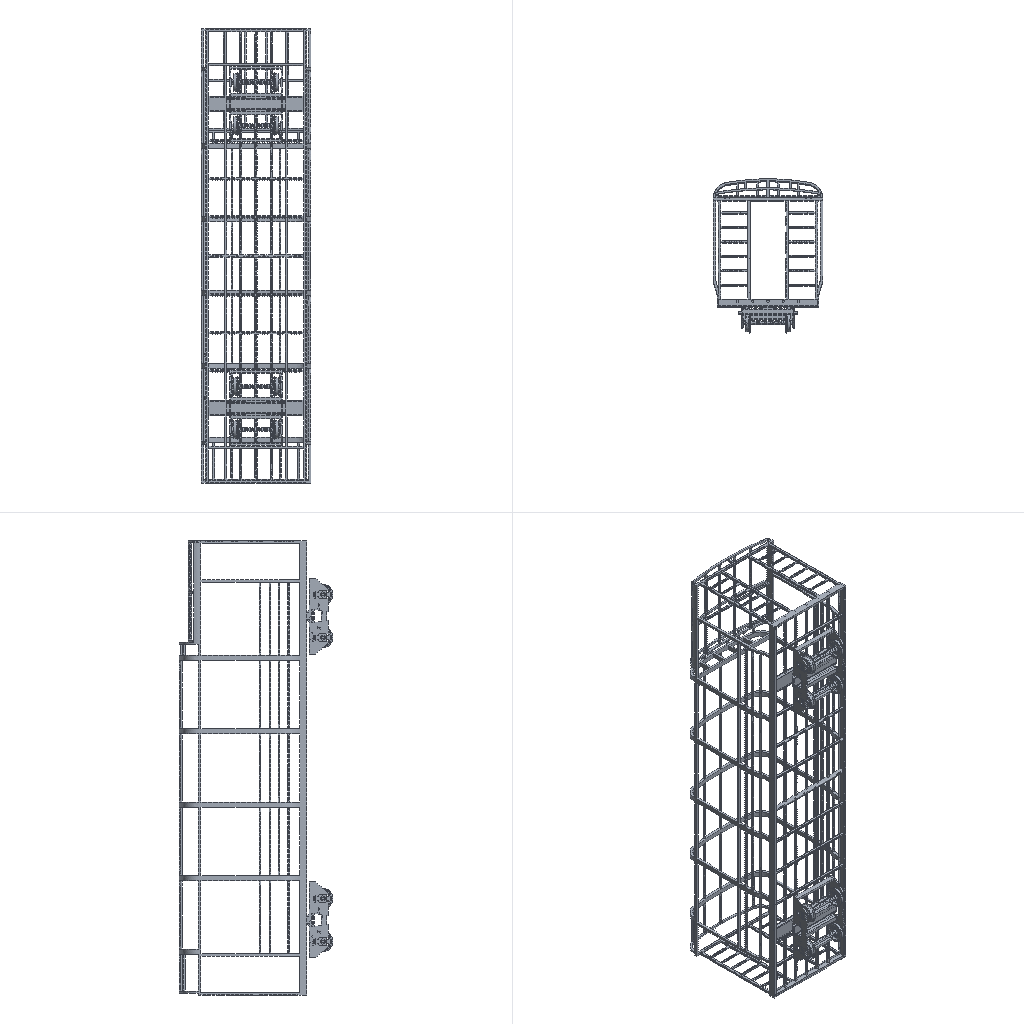Simulation study | ansys workbench
Set-up summary:
category,name,step,type,value,unit,region
solver,ansys_workbench
units,mm-N-s-tonne (MPa),,stated,"/units,MPA"
analysis,LS1,,static
load_step,LS1,LS1,static,nsubst=1; time=1
mesh,nodes,,,844920
mesh,elements,,,484857
element_type,SOLID187,,,440747
element_type,CONTA174,,,29118
element_type,TARGE170,,,10972
element_type,SOLID186,,,4020
material,Structural Steel,,E,200000,tonne s^-2 mm^-1
material,Structural Steel,,nu,0.3
material,Structural Steel,,density,7.85e-09,tonne mm^-3
material,Structural Steel,,conductivity,60.5,tonne mm s^-3 C^-1
material,Structural Steel,,specific_heat,4.34e+08,mm^2 s^-2 C^-1
material,Structural Steel,,cte,1.2e-05,C^-1
material,Structural Steel,,permeability,10000
material,Structural Steel,,resistivity,0.00017,ohm mm
load,,LS1,moment,"2.62e+06 [dir=(1, 0, 0) n=12]",,all
load,,LS1,force,"4284 [dir=(-1, 0, 0) n=3]",,all
load,ACEL,LS1,gravity (ACEL; gravity acts opposite),"9810.13 [dir=(0.02664, -0.9996, 0)]",,all
bc,Constant Zero Displacement X,model,fixed,[dofs=UX],,_DISPZEROUX
bc,Constant Zero Displacement Y,model,fixed,[dofs=UY],,_DISPZEROUY
bc,Constant Zero Displacement Z,model,fixed,[dofs=UZ],,_DISPZEROUZ
contact,Contact Region 10,,bonded (always),element=CONTA174
contact,Contact Region 11,,bonded (always),element=CONTA174
contact,Contact Region 12,,bonded (always),element=CONTA174
contact,Contact Region 13,,bonded (always),element=CONTA174
contact,Contact Region 14,,bonded (always),element=CONTA174
contact,Contact Region 15,,bonded (always),element=CONTA174
contact,Contact Region 16,,bonded (always),element=CONTA174
contact,Contact Region 17,,bonded (always),element=CONTA174
contact,Contact Region 18,,bonded (always),element=CONTA174
contact,Contact Region 19,,bonded (always),element=CONTA174
contact,Contact Region 20,,bonded (always),element=CONTA174
contact,Contact Region 21,,bonded (always),element=CONTA174
contact,Contact Region 22,,bonded (always),element=CONTA174
contact,Contact Region 23,,bonded (always),element=CONTA174
contact,Contact Region 24,,bonded (always),element=CONTA174
contact,Contact Region 25,,bonded (always),element=CONTA174
contact,Contact Region 26,,bonded (always),element=CONTA174
contact,Contact Region 27,,bonded (always),element=CONTA174
contact,Contact Region 28,,bonded (always),element=CONTA174
contact,Contact Region 29,,bonded (always),element=CONTA174
contact,Contact Region 30,,bonded (always),element=CONTA174
contact,Contact Region 31,,bonded (always),element=CONTA174
contact,Contact Region 32,,bonded (always),element=CONTA174
contact,Contact Region 33,,bonded (always),element=CONTA174
contact,Contact Region 34,,bonded (always),element=CONTA174
contact,Contact Region 35,,bonded (always),element=CONTA174
contact,Contact Region 36,,bonded (always),element=CONTA174
contact,Contact Region 37,,bonded (always),element=CONTA174
contact,Contact Region 38,,bonded (always),element=CONTA174
contact,Contact Region 39,,bonded (always),element=CONTA174
contact,Contact Region 40,,bonded (always),element=CONTA174
contact,Contact Region 41,,bonded (always),element=CONTA174
contact,Contact Region 42,,bonded (always),element=CONTA174
contact,Contact Region 43,,bonded (always),element=CONTA174
contact,Contact Region 44,,bonded (always),element=CONTA174
contact,Contact Region 45,,bonded (always),element=CONTA174
contact,Contact Region 46,,bonded (always),element=CONTA174
contact,Contact Region 47,,bonded (always),element=CONTA174
contact,Contact Region 48,,bonded (always),element=CONTA174
contact,Contact Region 49,,bonded (always),element=CONTA174
contact,Contact Region 50,,bonded (always),element=CONTA174
contact,Contact Region 51,,bonded (always),element=CONTA174
contact,Contact Region 52,,bonded (always),element=CONTA174
contact,Contact Region 53,,bonded (always),element=CONTA174
contact,Contact Region 54,,bonded (always),element=CONTA174
contact,Contact Region 55,,bonded (always),element=CONTA174
contact,Contact Region 56,,bonded (always),element=CONTA174
contact,Contact Region 57,,bonded (always),element=CONTA174
contact,Contact Region 58,,bonded (always),element=CONTA174
contact,Contact Region 59,,bonded (always),element=CONTA174
contact,Contact Region 60,,bonded (always),element=CONTA174
contact,Contact Region 61,,bonded (always),element=CONTA174
contact,Contact Region 62,,bonded (always),element=CONTA174
contact,Contact Region 63,,bonded (always),element=CONTA174
contact,Contact Region 64,,bonded (always),element=CONTA174
contact,Contact Region 65,,bonded (always),element=CONTA174
contact,Contact Region 66,,bonded (always),element=CONTA174
contact,Contact Region 67,,bonded (always),element=CONTA174
contact,Contact Region 68,,bonded (always),element=CONTA174
contact,Contact Region 69,,bonded (always),element=CONTA174
contact,Contact Region 70,,bonded (always),element=CONTA174
contact,Contact Region 71,,bonded (always),element=CONTA174
contact,Contact Region 72,,bonded (always),element=CONTA174
contact,Contact Region 73,,bonded (always),element=CONTA174
contact,Contact Region 74,,bonded (always),element=CONTA174
contact,Contact Region 75,,bonded (always),element=CONTA174
contact,Contact Region 76,,bonded (always),element=CONTA174
contact,Contact Region 77,,bonded (always),element=CONTA174
contact,Contact Region 78,,bonded (always),element=CONTA174
contact,Contact Region 79,,bonded (always),element=CONTA174
contact,Contact Region 80,,bonded (always),element=CONTA174
contact,Contact Region 81,,bonded (always),element=CONTA174
contact,Contact Region 82,,bonded (always),element=CONTA174
contact,Contact Region 83,,bonded (always),element=CONTA174
contact,Contact Region 84,,bonded (always),element=CONTA174
contact,Contact Region 85,,bonded (always),element=CONTA174
contact,Contact Region 86,,bonded (always),element=CONTA174
contact,Contact Region 87,,bonded (always),element=CONTA174
contact,Contact Region 88,,bonded (always),element=CONTA174
contact,Contact Region 89,,bonded (always),element=CONTA174
contact,Contact Region 90,,bonded (always),element=CONTA174
contact,Contact Region 91,,bonded (always),element=CONTA174
contact,Contact Region 92,,bonded (always),element=CONTA174
contact,Contact Region 93,,bonded (always),element=CONTA174
contact,Contact Region 94,,bonded (always),element=CONTA174
contact,Contact Region 95,,bonded (always),element=CONTA174
contact,Contact Region 96,,bonded (always),element=CONTA174
contact,Contact Region 97,,bonded (always),element=CONTA174
contact,Contact Region 98,,bonded (always),element=CONTA174
contact,Contact Region 99,,bonded (always),element=CONTA174
contact,Contact Region 100,,bonded (always),element=CONTA174
contact,Contact Region 101,,bonded (always),element=CONTA174
contact,Contact Region 102,,bonded (always),element=CONTA174
contact,Contact Region 103,,bonded (always),element=CONTA174
contact,Contact Region 104,,bonded (always),element=CONTA174
contact,Contact Region 105,,bonded (always),element=CONTA174
contact,Contact Region 106,,bonded (always),element=CONTA174
contact,Contact Region 107,,bonded (always),element=CONTA174
contact,Contact Region 108,,bonded (always),element=CONTA174
contact,Contact Region 109,,bonded (always),element=CONTA174
contact,Contact Region 110,,bonded (always),element=CONTA174
contact,Contact Region 111,,bonded (always),element=CONTA174
contact,Contact Region 112,,bonded (always),element=CONTA174
contact,Contact Region 113,,bonded (always),element=CONTA174
contact,Contact Region 114,,bonded (always),element=CONTA174
contact,Contact Region 115,,bonded (always),element=CONTA174
contact,Contact Region 116,,bonded (always),element=CONTA174
contact,Contact Region 117,,bonded (always),element=CONTA174
contact,Contact Region 118,,bonded (always),element=CONTA174
contact,Contact Region 119,,bonded (always),element=CONTA174
contact,Contact Region 120,,bonded (always),element=CONTA174
contact,contact 112,,bonded (always),element=CONTA174
contact,contact 113,,bonded (always),element=CONTA174
contact,contact 114,,bonded (always),element=CONTA174
contact,contact 115,,bonded (always),element=CONTA174
contact,contact 116,,bonded (always),element=CONTA174
contact,contact 117,,bonded (always),element=CONTA174
contact,contact 118,,bonded (always),element=CONTA174
named_set,_DISPZEROUX,,node,2976
named_set,_DISPZEROUY,,node,2976
named_set,_DISPZEROUZ,,node,1488
Ansys APDL input file, long lists of numbers shortened:
/batch
/config,noeldb,1     ! force off writing results to database
*get,_wallstrt,active,,time,wall
! ANSYS input file written by Workbench version 2021 R1
! File used for geometry attach:
/title,_______--____ 2 (C5)
! ****** Begin Custom Load Command Snippet ******
/COM, ACT Extensions:
/COM,     LSDYNA, 2021.1
/COM,
! ****** End   Custom Load Command Snippet ******
*DIM,_wb_ProjectScratch_dir,string,248
_wb_ProjectScratch_dir(1) = ''
*DIM,_wb_SolverFiles_dir,string,248
_wb_SolverFiles_dir(1) = ''
*DIM,_wb_userfiles_dir,string,248
_wb_userfiles_dir(1) = ''
/com,--- Data in consistent NMM units. See Solving Units in the help system for more information.
/units,MPA
/nopr
/wb,file,start              !  signify a WB generated input file
/prep7
! Turn off shape checking because checks already performed inside WB mesher.
! See help system for more information.
SHPP,OFF,,NOWARN
/nolist
etcon,set             ! allow ANSYS to choose best KEYOP's for 180x elements, resets any applicable keyopt to MAPDL defaults
/com,*********** Nodes for the whole assembly ***********
nblock,3,,929390
(1i9,3e20.9e3)
        1     5.000000000E+02    -2.700000000E+02     8.500000000E+01
! (844899 more lines like these left out)
-1
/com,*********** Nodes for all Remote Points ***********
nblock,3
(1i9,3e20.9e3)
   844901     0.000000000E+00    -4.570000000E+02     1.250000000E+03
! (19 more lines like these left out)
-1
/wb,elem,start            !  set before creation of elements
/com,*********** Elements for Body 1 "____-0|NONE" ***********
et,1,187
eblock,19,solid,,219008
(19i9)
        1        1        1        1        0        0        0        0       10        0   225760   496373   499028   502293   501893   835194   841376   835201   835199
! (438015 more lines like these left out)
-1
/com,*********** Elements for Body 2 "______|NONE" ***********
et,2,186
keyo,2,2,1          ! set full integration on SOLID186
eblock,19,solid,,316
(19i9)
        2        2        2        2        0        0        0        0       20        0      914     6556     6586     6589     6565     6931     6901     6898     6922
! (631 more lines like these left out)
-1
/com,*********** Elements for Body 3 "______|NONE[2]" ***********
et,3,186
keyo,3,2,1          ! set full integration on SOLID186
eblock,19,solid,,316
(19i9)
        3        3        3        3        0        0        0        0       20        0     1663    12147    12177    12180    12156    12522    12492    12489    12513
! (631 more lines like these left out)
-1
/com,*********** Elements for Body 4 "______|NONE[3]" ***********
et,4,186
keyo,4,2,1          ! set full integration on SOLID186
eblock,19,solid,,420
(19i9)
        4        4        4        4        0        0        0        0       20        0     1243     9304     9447     9466     9364     9345     9446     9485     9365
! (839 more lines like these left out)
-1
/com,*********** Elements for Body 5 "______|NONE[4]" ***********
et,5,186
keyo,5,2,1          ! set full integration on SOLID186
eblock,19,solid,,420
(19i9)
        5        5        5        5        0        0        0        0       20        0      481     3579     3722     3741     3639     3620     3721     3760     3640
! (839 more lines like these left out)
-1
! (55 more sections like these left out)
/wb,elem,end               !  done creating elements
/com,*********** Send User Defined Coordinate System(s) ***********
csys,0
toffst,273.15,  ! Temperature offset from absolute zero
/com,*********** Set Reference Temperature ***********
tref,22.
/wb,mat,start              !  starting to send materials
/com,*********** Send Materials ***********
Temperature = 'TEMP' ! Temperature
MP,DENS,1,7.85e-09,	! tonne mm^-3
MP,ALPX,1,1.2e-05,	! C^-1
MP,C,1,434000000,	! mm^2 s^-2 C^-1
MP,KXX,1,60.5,	! tonne mm s^-3 C^-1
MP,RSVX,1,0.00017,	! ohm mm
MP,EX,1,200000,	! tonne s^-2 mm^-1
MP,NUXY,1,0.3,
MP,MURX,1,10000,
Temperature = 'TEMP' ! Temperature
MP,DENS,2,7.85e-09,	! tonne mm^-3
MP,ALPX,2,1.2e-05,	! C^-1
MP,C,2,434000000,	! mm^2 s^-2 C^-1
MP,KXX,2,60.5,	! tonne mm s^-3 C^-1
MP,RSVX,2,0.00017,	! ohm mm
MP,EX,2,200000,	! tonne s^-2 mm^-1
MP,NUXY,2,0.3,
MP,MURX,2,10000,
Temperature = 'TEMP' ! Temperature
MP,DENS,3,7.85e-09,	! tonne mm^-3
MP,ALPX,3,1.2e-05,	! C^-1
MP,C,3,434000000,	! mm^2 s^-2 C^-1
MP,KXX,3,60.5,	! tonne mm s^-3 C^-1
MP,RSVX,3,0.00017,	! ohm mm
MP,EX,3,200000,	! tonne s^-2 mm^-1
MP,NUXY,3,0.3,
MP,MURX,3,10000,
Temperature = 'TEMP' ! Temperature
MP,DENS,4,7.85e-09,	! tonne mm^-3
MP,ALPX,4,1.2e-05,	! C^-1
MP,C,4,434000000,	! mm^2 s^-2 C^-1
MP,KXX,4,60.5,	! tonne mm s^-3 C^-1
MP,RSVX,4,0.00017,	! ohm mm
MP,EX,4,200000,	! tonne s^-2 mm^-1
MP,NUXY,4,0.3,
MP,MURX,4,10000,
Temperature = 'TEMP' ! Temperature
MP,DENS,5,7.85e-09,	! tonne mm^-3
MP,ALPX,5,1.2e-05,	! C^-1
MP,C,5,434000000,	! mm^2 s^-2 C^-1
MP,KXX,5,60.5,	! tonne mm s^-3 C^-1
MP,RSVX,5,0.00017,	! ohm mm
MP,EX,5,200000,	! tonne s^-2 mm^-1
MP,NUXY,5,0.3,
MP,MURX,5,10000,
Temperature = 'TEMP' ! Temperature
MP,DENS,6,7.85e-09,	! tonne mm^-3
MP,ALPX,6,1.2e-05,	! C^-1
MP,C,6,434000000,	! mm^2 s^-2 C^-1
MP,KXX,6,60.5,	! tonne mm s^-3 C^-1
MP,RSVX,6,0.00017,	! ohm mm
MP,EX,6,200000,	! tonne s^-2 mm^-1
MP,NUXY,6,0.3,
MP,MURX,6,10000,
Temperature = 'TEMP' ! Temperature
MP,DENS,7,7.85e-09,	! tonne mm^-3
MP,ALPX,7,1.2e-05,	! C^-1
MP,C,7,434000000,	! mm^2 s^-2 C^-1
MP,KXX,7,60.5,	! tonne mm s^-3 C^-1
MP,RSVX,7,0.00017,	! ohm mm
MP,EX,7,200000,	! tonne s^-2 mm^-1
MP,NUXY,7,0.3,
MP,MURX,7,10000,
Temperature = 'TEMP' ! Temperature
MP,DENS,8,7.85e-09,	! tonne mm^-3
MP,ALPX,8,1.2e-05,	! C^-1
MP,C,8,434000000,	! mm^2 s^-2 C^-1
MP,KXX,8,60.5,	! tonne mm s^-3 C^-1
MP,RSVX,8,0.00017,	! ohm mm
MP,EX,8,200000,	! tonne s^-2 mm^-1
MP,NUXY,8,0.3,
MP,MURX,8,10000,
Temperature = 'TEMP' ! Temperature
MP,DENS,9,7.85e-09,	! tonne mm^-3
MP,ALPX,9,1.2e-05,	! C^-1
MP,C,9,434000000,	! mm^2 s^-2 C^-1
MP,KXX,9,60.5,	! tonne mm s^-3 C^-1
MP,RSVX,9,0.00017,	! ohm mm
MP,EX,9,200000,	! tonne s^-2 mm^-1
! (461 more lines like these left out)
/wb,mat,end                !  done sending materials
!************************* Model Summary ********************
!____-0|NONE,	结构钢,	matid,	1
!______|NONE,	结构钢,	matid,	2
!______|NONE[2],	结构钢,	matid,	3
! (59 more lines like these left out)
*get,_xmin,node,,mnloc,x
*get,_ymin,node,,mnloc,y
*get,_zmin,node,,mnloc,z
*get,_xmax,node,,mxloc,x
*get,_ymax,node,,mxloc,y
*get,_zmax,node,,mxloc,z
_ASMDIAG=(_xmax-_xmin)*(_xmax-_xmin)+(_ymax-_ymin)*(_ymax-_ymin)+(_zmax-_zmin)*(_zmax-_zmin)
_ASMDIAG=SQRT(_ASMDIAG)
/wb,contact,start          !  starting to send contact
/com,*********** Create Contact "接触区域 10" ***********
/com,            Real Constant Set For Above Contact Is 62 & 61
*set,tid,62
*set,cid,61
r,tid
r,cid
et,tid,170
et,cid,174
eblock,10,,,42
(15i9)
   662848       62       62       62        0     6714     6723     6734     6734     7990     8015     6734     7992
! (41 more lines like these left out)
-1
eblock,10,,,42
(15i9)
   662890       61       61       61        0     6714     6723     6734     6734     7990     8015     6734     7992
! (41 more lines like these left out)
-1
eblock,10,,,21
(15i9)
   662932       61       62       61        0     9885    10045     9244     9244    11813    10203     9244    10202
! (20 more lines like these left out)
-1
eblock,10,,,21
(15i9)
   662953       62       61       62        0     9885    10045     9244     9244    11813    10203     9244    10202
! (20 more lines like these left out)
-1
keyo,cid,8,2               ! auto create asymmetric contact (from Program Controlled setting)
keyo,cid,10,0              ! adjust contact stiffness each NR iteration (from Program Controlled setting)
keyo,cid,12,5              ! bonded always
keyo,cid,18,1              ! small sliding turned on by application
keyo,cid,2,0               ! augmented Lagrange (from Program Controlled setting)
keyo,cid,4,0               ! on Gauss point (from Program Controlled setting)
keyo,cid,9,1               ! ignore initial gaps/penetration
keyo,cid,7,0               ! No Prediction
rmod,tid,3,10.      ! FKN
rmod,tid,5,0.       ! ICONT
rmod,tid,6,0.       ! PINB
rmod,tid,10,0.      ! CNOF
rmod,tid,12,0.      ! FKT
rmod,tid,36,14962   ! WB DSID
rmod,cid,3,10.      ! FKN
rmod,cid,5,0.       ! ICONT
rmod,cid,6,0.       ! PINB
rmod,cid,10,0.      ! CNOF
rmod,cid,12,0.      ! FKT
rmod,cid,36,14962   ! WB DSID
/com,*********** Create Contact "接触区域 11" ***********
/com,            Real Constant Set For Above Contact Is 64 & 63
*set,tid,64
*set,cid,63
r,tid
r,cid
et,tid,170
et,cid,174
eblock,10,,,48
(15i9)
   662974       64       64       64        0     6688     6733     6595     6595     7938     7613     6595     7610
! (47 more lines like these left out)
-1
eblock,10,,,48
(15i9)
   663022       63       63       63        0     6688     6733     6595     6595     7938     7613     6595     7610
! (47 more lines like these left out)
-1
eblock,10,,,21
(15i9)
   663070       63       64       63        0     3534     3522     3523     3523     4485     4484     3523     4488
! (20 more lines like these left out)
-1
eblock,10,,,21
(15i9)
   663091       64       63       64        0     3534     3522     3523     3523     4485     4484     3523     4488
! (20 more lines like these left out)
-1
keyo,cid,8,2               ! auto create asymmetric contact (from Program Controlled setting)
keyo,cid,10,0              ! adjust contact stiffness each NR iteration (from Program Controlled setting)
keyo,cid,12,5              ! bonded always
keyo,cid,18,1              ! small sliding turned on by application
keyo,cid,2,0               ! augmented Lagrange (from Program Controlled setting)
keyo,cid,4,0               ! on Gauss point (from Program Controlled setting)
keyo,cid,9,1               ! ignore initial gaps/penetration
keyo,cid,7,0               ! No Prediction
rmod,tid,3,10.      ! FKN
rmod,tid,5,0.       ! ICONT
rmod,tid,6,0.       ! PINB
rmod,tid,10,0.      ! CNOF
rmod,tid,12,0.      ! FKT
rmod,tid,36,14965   ! WB DSID
rmod,cid,3,10.      ! FKN
rmod,cid,5,0.       ! ICONT
rmod,cid,6,0.       ! PINB
rmod,cid,10,0.      ! CNOF
rmod,cid,12,0.      ! FKT
rmod,cid,36,14965   ! WB DSID
/com,*********** Create Contact "接触区域 12" ***********
/com,            Real Constant Set For Above Contact Is 66 & 65
*set,tid,66
*set,cid,65
r,tid
r,cid
et,tid,170
et,cid,174
eblock,10,,,16
(15i9)
   663112       66       66       66        0     6741     6708     6696     6709     7977     7955     7956     7980
! (15 more lines like these left out)
-1
eblock,10,,,16
(15i9)
   663128       65       65       65        0     6741     6708     6696     6709     7977     7955     7956     7980
! (15 more lines like these left out)
-1
eblock,10,,,12
(15i9)
   663144       65       66       65        0     1744     1745     1761     1756     2255     2259     2289     2257
! (11 more lines like these left out)
-1
eblock,10,,,12
(15i9)
   663156       66       65       66        0     1744     1745     1761     1756     2255     2259     2289     2257
! (11 more lines like these left out)
-1
keyo,cid,8,2               ! auto create asymmetric contact (from Program Controlled setting)
keyo,cid,10,0              ! adjust contact stiffness each NR iteration (from Program Controlled setting)
keyo,cid,12,5              ! bonded always
keyo,cid,18,1              ! small sliding turned on by application
keyo,cid,2,0               ! augmented Lagrange (from Program Controlled setting)
keyo,cid,4,0               ! on Gauss point (from Program Controlled setting)
keyo,cid,9,1               ! ignore initial gaps/penetration
keyo,cid,7,0               ! No Prediction
rmod,tid,3,10.      ! FKN
rmod,tid,5,0.       ! ICONT
rmod,tid,6,0.       ! PINB
rmod,tid,10,0.      ! CNOF
rmod,tid,12,0.      ! FKT
rmod,tid,36,14968   ! WB DSID
rmod,cid,3,10.      ! FKN
rmod,cid,5,0.       ! ICONT
rmod,cid,6,0.       ! PINB
rmod,cid,10,0.      ! CNOF
rmod,cid,12,0.      ! FKT
rmod,cid,36,14968   ! WB DSID
/com,*********** Create Contact "接触区域 13" ***********
/com,            Real Constant Set For Above Contact Is 68 & 67
*set,tid,68
*set,cid,67
r,tid
r,cid
et,tid,170
et,cid,174
eblock,10,,,15
(15i9)
   663168       68       68       68        0     6738     6691     6692     6739     7945     7944     7948     8042
! (14 more lines like these left out)
-1
eblock,10,,,15
(15i9)
   663183       67       67       67        0     6738     6691     6692     6739     7945     7944     7948     8042
! (14 more lines like these left out)
-1
eblock,10,,,12
(15i9)
   663198       67       68       67        0       21       16        4        5      549      517      515      519
! (11 more lines like these left out)
-1
eblock,10,,,12
(15i9)
   663210       68       67       68        0       21       16        4        5      549      517      515      519
! (11 more lines like these left out)
-1
keyo,cid,8,2               ! auto create asymmetric contact (from Program Controlled setting)
keyo,cid,10,0              ! adjust contact stiffness each NR iteration (from Program Controlled setting)
keyo,cid,12,5              ! bonded always
keyo,cid,18,1              ! small sliding turned on by application
keyo,cid,2,0               ! augmented Lagrange (from Program Controlled setting)
keyo,cid,4,0               ! on Gauss point (from Program Controlled setting)
keyo,cid,9,1               ! ignore initial gaps/penetration
keyo,cid,7,0               ! No Prediction
rmod,tid,3,10.      ! FKN
rmod,tid,5,0.       ! ICONT
rmod,tid,6,0.       ! PINB
rmod,tid,10,0.      ! CNOF
rmod,tid,12,0.      ! FKT
rmod,tid,36,14971   ! WB DSID
rmod,cid,3,10.      ! FKN
rmod,cid,5,0.       ! ICONT
rmod,cid,6,0.       ! PINB
rmod,cid,10,0.      ! CNOF
rmod,cid,12,0.      ! FKT
rmod,cid,36,14971   ! WB DSID
/com,*********** Create Contact "接触区域 14" ***********
/com,            Real Constant Set For Above Contact Is 70 & 69
*set,tid,70
*set,cid,69
r,tid
r,cid
et,tid,170
et,cid,174
eblock,10,,,33
(15i9)
   663222       70       70       70        0     7129     7127     7128     7133     8908     8907     8909     8911
! (32 more lines like these left out)
-1
eblock,10,,,33
(15i9)
   663255       69       69       69        0     7129     7127     7128     7133     8908     8907     8909     8911
! (32 more lines like these left out)
-1
eblock,10,,,170
(15i9)
   663288       69       70       69        0    17468    17488    17473    17473    26290    26306    17473    26287
! (169 more lines like these left out)
-1
eblock,10,,,170
(15i9)
   663458       70       69       70        0    17468    17488    17473    17473    26290    26306    17473    26287
! (169 more lines like these left out)
-1
keyo,cid,8,2               ! auto create asymmetric contact (from Program Controlled setting)
keyo,cid,10,0              ! adjust contact stiffness each NR iteration (from Program Controlled setting)
keyo,cid,12,5              ! bonded always
keyo,cid,18,1              ! small sliding turned on by application
keyo,cid,2,0               ! augmented Lagrange (from Program Controlled setting)
keyo,cid,4,0               ! on Gauss point (from Program Controlled setting)
keyo,cid,9,1               ! ignore initial gaps/penetration
keyo,cid,7,0               ! No Prediction
rmod,tid,3,10.      ! FKN
rmod,tid,5,0.       ! ICONT
rmod,tid,6,0.       ! PINB
rmod,tid,10,0.      ! CNOF
rmod,tid,12,0.      ! FKT
rmod,tid,36,14974   ! WB DSID
rmod,cid,3,10.      ! FKN
rmod,cid,5,0.       ! ICONT
rmod,cid,6,0.       ! PINB
rmod,cid,10,0.      ! CNOF
rmod,cid,12,0.      ! FKT
rmod,cid,36,14974   ! WB DSID
! (106 more sections like these left out)
/wb,contact,end            !  done creating contacts
/golist
/wb,load,start             !  starting to send loads
/com,******* Constant Zero Displacement X *******
CMBLOCK,_DISPZEROUX,NODE,     2976
(8i10)
     33525     33526     33527     33528     33529     33530     33531     33532
! (371 more lines like these left out)
cmsel,s,_DISPZEROUX
d,all,ux,0
nsel,all
/com,******* Constant Zero Displacement Y *******
CMBLOCK,_DISPZEROUY,NODE,     2976
(8i10)
     33525     33526     33527     33528     33529     33530     33531     33532
! (371 more lines like these left out)
cmsel,s,_DISPZEROUY
d,all,uy,0
nsel,all
/com,******* Constant Zero Displacement Z *******
CMBLOCK,_DISPZEROUZ,NODE,     1488
(8i10)
     33525     33526     33527     33528     33529     33530     33531     33532
! (185 more lines like these left out)
cmsel,s,_DISPZEROUZ
d,all,uz,0
nsel,all
/com,*********** Create Remote Point "内部远程点" ***********
! -------- Remote Point Used by "力矩" --------
*set,tid,284
*set,cid,283
et,cid,174
et,tid,170
keyo,tid,2,1               ! Don't fix the pilot node
keyo,tid,4,0               ! Activate all DOF's due to large deformation
keyo,cid,12,5              ! Bonded Contact
keyo,cid,4,1               ! Deformable RBE3 style load
keyo,cid,2,2               ! MPC style contact
eblock,10,,,358
(15i9)
   684792      283      283      283        0    38713    38614    38728    38728    39254    39255    38728    40038
! (357 more lines like these left out)
-1
*set,_npilot,844905
_npilot15320=_npilot
type,tid
mat ,cid
real,cid
tshape,pilo
en,685150,_npilot
tshape
/com,*********** Create Remote Point "内部远程点 2" ***********
! -------- Remote Point Used by "力矩 2" --------
*set,tid,286
*set,cid,285
et,cid,174
et,tid,170
keyo,tid,2,1               ! Don't fix the pilot node
keyo,tid,4,0               ! Activate all DOF's due to large deformation
keyo,cid,12,5              ! Bonded Contact
keyo,cid,4,1               ! Deformable RBE3 style load
keyo,cid,2,2               ! MPC style contact
eblock,10,,,360
(15i9)
   685151      285      285      285        0    71272    71189    71399    71399    72063    72066    71399    72735
! (359 more lines like these left out)
-1
*set,_npilot,844906
_npilot15323=_npilot
type,tid
mat ,cid
real,cid
tshape,pilo
en,685511,_npilot
tshape
/com,*********** Create Remote Point "内部远程点 3" ***********
! -------- Remote Point Used by "力矩 3" --------
*set,tid,288
*set,cid,287
et,cid,174
et,tid,170
keyo,tid,2,1               ! Don't fix the pilot node
keyo,tid,4,0               ! Activate all DOF's due to large deformation
keyo,cid,12,5              ! Bonded Contact
keyo,cid,4,1               ! Deformable RBE3 style load
keyo,cid,2,2               ! MPC style contact
eblock,10,,,358
(15i9)
   685512      287      287      287        0    27853    27754    27868    27868    28394    28395    27868    29178
! (357 more lines like these left out)
-1
*set,_npilot,844907
_npilot15326=_npilot
type,tid
mat ,cid
real,cid
tshape,pilo
en,685870,_npilot
tshape
/com,*********** Create Remote Point "内部远程点 4" ***********
! -------- Remote Point Used by "力矩 4" --------
*set,tid,290
*set,cid,289
et,cid,174
et,tid,170
keyo,tid,2,1               ! Don't fix the pilot node
keyo,tid,4,0               ! Activate all DOF's due to large deformation
keyo,cid,12,5              ! Bonded Contact
keyo,cid,4,1               ! Deformable RBE3 style load
keyo,cid,2,2               ! MPC style contact
eblock,10,,,360
(15i9)
   685871      289      289      289        0    60036    59953    60163    60163    60827    60830    60163    61499
! (359 more lines like these left out)
-1
*set,_npilot,844908
_npilot15329=_npilot
type,tid
mat ,cid
real,cid
tshape,pilo
en,686231,_npilot
tshape
/com,*********** Create Remote Point "内部远程点 17" ***********
! -------- Remote Point Used by "点质量" --------
*set,tid,292
*set,cid,291
et,cid,174
et,tid,170
keyo,tid,2,1               ! Don't fix the pilot node
keyo,tid,4,0               ! Activate all DOF's due to large deformation
keyo,cid,12,5              ! Bonded Contact
keyo,cid,4,1               ! Deformable RBE3 style load
keyo,cid,2,2               ! MPC style contact
eblock,10,,,6072
(15i9)
   686232      291      291      291        0   148608   149004   149355   149355   346755   349666   149355   346758
! (6071 more lines like these left out)
-1
*set,_npilot,844917
_npilot15533=_npilot
type,tid
mat ,cid
real,cid
tshape,pilo
en,692304,_npilot
tshape
! (2 more sections like these left out)
/com,*********** Construct Moment Using Remote Attachment ***********
/com,*********** Construct Moment Using Remote Attachment ***********
*DIM,_loadvari15322x,TABLE,2,1,1,TIME,
! Time values
_loadvari15322x(1,0,1) = 0.
_loadvari15322x(2,0,1) = 1.
! Load values
_loadvari15322x(1,1,1) = 0.
_loadvari15322x(2,1,1) = 655000.
*DIM,_loadvari15322y,TABLE,2,1,1,TIME,
! Time values
_loadvari15322y(1,0,1) = 0.
_loadvari15322y(2,0,1) = 1.
! Load values
_loadvari15322y(1,1,1) = 0.
_loadvari15322y(2,1,1) = 0.
*DIM,_loadvari15322z,TABLE,2,1,1,TIME,
! Time values
_loadvari15322z(1,0,1) = 0.
_loadvari15322z(2,0,1) = 1.
! Load values
_loadvari15322z(1,1,1) = 0.
_loadvari15322z(2,1,1) = 0.
/com,*********** Construct Moment Using Remote Attachment ***********
*DIM,_loadvari15325x,TABLE,2,1,1,TIME,
! Time values
_loadvari15325x(1,0,1) = 0.
_loadvari15325x(2,0,1) = 1.
! Load values
_loadvari15325x(1,1,1) = 0.
_loadvari15325x(2,1,1) = 655000.
*DIM,_loadvari15325y,TABLE,2,1,1,TIME,
! Time values
_loadvari15325y(1,0,1) = 0.
_loadvari15325y(2,0,1) = 1.
! Load values
_loadvari15325y(1,1,1) = 0.
_loadvari15325y(2,1,1) = 0.
*DIM,_loadvari15325z,TABLE,2,1,1,TIME,
! Time values
_loadvari15325z(1,0,1) = 0.
_loadvari15325z(2,0,1) = 1.
! Load values
_loadvari15325z(1,1,1) = 0.
_loadvari15325z(2,1,1) = 0.
/com,*********** Construct Moment Using Remote Attachment ***********
*DIM,_loadvari15328x,TABLE,2,1,1,TIME,
! Time values
_loadvari15328x(1,0,1) = 0.
_loadvari15328x(2,0,1) = 1.
! Load values
_loadvari15328x(1,1,1) = 0.
_loadvari15328x(2,1,1) = 655000.
*DIM,_loadvari15328y,TABLE,2,1,1,TIME,
! Time values
_loadvari15328y(1,0,1) = 0.
_loadvari15328y(2,0,1) = 1.
! Load values
_loadvari15328y(1,1,1) = 0.
_loadvari15328y(2,1,1) = 0.
*DIM,_loadvari15328z,TABLE,2,1,1,TIME,
! Time values
_loadvari15328z(1,0,1) = 0.
_loadvari15328z(2,0,1) = 1.
! Load values
_loadvari15328z(1,1,1) = 0.
_loadvari15328z(2,1,1) = 0.
/com,*********** Construct Remote Force ***********
*DIM,_loadvari15589x,TABLE,2,1,1,TIME,
! Time values
_loadvari15589x(1,0,1) = 0.
_loadvari15589x(2,0,1) = 1.
! Load values
_loadvari15589x(1,1,1) = 0.
_loadvari15589x(2,1,1) = -4284.
*DIM,_loadvari15589y,TABLE,2,1,1,TIME,
! Time values
_loadvari15589y(1,0,1) = 0.
_loadvari15589y(2,0,1) = 1.
! Load values
_loadvari15589y(1,1,1) = 0.
_loadvari15589y(2,1,1) = 0.
*DIM,_loadvari15589z,TABLE,2,1,1,TIME,
! Time values
_loadvari15589z(1,0,1) = 0.
_loadvari15589z(2,0,1) = 1.
! Load values
_loadvari15589z(1,1,1) = 0.
_loadvari15589z(2,1,1) = 0.
/com,*********** Construct Remote Mass Using Remote Attachment ***********
*set,_tid,297
et,_tid,21           ! MASS21 element
type,_tid
mat ,_tid
real,_tid
keyo,_tid,3,2        ! 3d mass without rotary inertia
r,_tid,2.8
en,702945,844917
/com,*********** Construct Remote Mass Using Remote Attachment ***********
*set,_tid,298
et,_tid,21           ! MASS21 element
type,_tid
mat ,_tid
real,_tid
keyo,_tid,3,2        ! 3d mass without rotary inertia
r,_tid,0.45
en,702946,844918
/gst,on,on
fini
*get,_numnode,node,0,count
*get,_numelem,elem,0,count
*get, _MAXELEMNUM, elem, 0, NUM, MAX
*get, _MAXNODENUM, node, 0, NUM, MAX
*get, _MAXELEMTYPE, etyp, 0, NUM, MAX
*get, _MAXREALCONST, real, 0, NUM, MAX
/go
/wb,load,end               !  done creating loads
/com,--- Number of total nodes = %_numnode%
/com,--- Number of contact elements = 40090
/com,--- Number of spring elements = 0
/com,--- Number of bearing elements = 0
/com,--- Number of solid elements = 444767
/com,--- Number of condensed parts = 0
/com,--- Number of total elements = %_numelem%
*get,_wallbsol,active,,time,wall
/com,****************************************************************************
/com,*************************    SOLUTION       ********************************
/com,****************************************************************************
/solu
antype,0                   ! static analysis
nlgeom,on                  ! Turn on Large Deformation Effects
_thickRatio=0.1     ! Ratio of thick parts in the model
eqsl,sparse,,,,,1
cntr,print,1               ! print out contact info and also make no initial contact an error
cntr,out,yes               ! write contact output to file.cmn due to many contact pairs present
dmpoption,emat,no             ! Don't combine emat file for DANSYS
dmpoption,esav,no             ! Don't combine esav file for DANSYS
nldiag,cont,iter           ! print out contact info each equilibrium iteration
rescontrol,define,last,last,,dele	   ! Program Controlled
/com,****************************************************
/com,******************* SOLVE FOR LS 1 OF 1 ****************
nsel,s,node,,844905
f,all,mx,655000.
f,all,my,0.
f,all,mz,0.
nsel,s,node,,844906
f,all,mx,%_loadvari15322x%
f,all,my,%_loadvari15322y%
f,all,mz,%_loadvari15322z%
nsel,s,node,,844907
f,all,mx,%_loadvari15325x%
f,all,my,%_loadvari15325y%
f,all,mz,%_loadvari15325z%
nsel,s,node,,844908
f,all,mx,%_loadvari15328x%
f,all,my,%_loadvari15328y%
f,all,mz,%_loadvari15328z%
nsel,all
nsel,s,node,,844920
f,all,fx,%_loadvari15589x%
f,all,fy,%_loadvari15589y%
f,all,fz,%_loadvari15589z%
nsel,all
acel,-261.3,9806.65,0.
/nopr
/gopr
/nolist
autots,on                  ! Workbench Program Controlled automatic time stepping
nsub,1,10,1                ! due to presence of general nonlinear
time,1.
outres,erase
outres,all,none
outres,nsol,all,
outres,rsol,all
outres,eangl,all
outres,etmp,all
outres,veng,all
outres,strs,all,
outres,epel,all,
outres,eppl,all,
outres,cont,all,
! *********** WB SOLVE COMMAND ***********
! check interactive state
*get,ANSINTER_,active,,int
*if,ANSINTER_,ne,0,then
/eof
*endif
solve
/com *************** Write FE CONNECTORS *********
CEWRITE,file,ce,,INTE
/com,****************************************************
/com,*************** FINISHED SOLVE FOR LS 1 *************
*get,_wallasol,active,,time,wall
/nopr
*get,_numnode,node,0,count
*get,_numelem,elem,0,count
*get, _MAXELEMNUM, elem, 0, NUM, MAX
*get, _MAXNODENUM, node, 0, NUM, MAX,,,INTERNAL
*get, _MAXELEMTYPE, etyp, 0, NUM, MAX
*get, _MAXREALCONST, real, 0, NUM, MAX
/gopr
/post1
xmlo,ENCODING,ISO-8859-1
xmlo,parm
/xml,parm,xml
fini
/gopr
*get,_walldone,active,,time,wall
_preptime=(_wallbsol-_wallstrt)*3600
_solvtime=(_wallasol-_wallbsol)*3600
_posttime=(_walldone-_wallasol)*3600
_totaltim=(_walldone-_wallstrt)*3600
*get,_dlbratio,active,0,solu,dlbr
*get,_combtime,active,0,solu,comb
/com,--- Total number of nodes = %_numnode%
/com,--- Total number of elements = %_numelem%
/com,--- Element load balance ratio = %_dlbratio%
/com,--- Time to combine distributed files = %_combtime%
/wb,file,end               ! done with WB generated input
Results summary:
result,analyses[0].index,,,1
result,analyses[0].system,,,SYS-2
result,analyses[0].deck,,,deck.dat
result,analyses[0].solve_status,,,completed
result,analyses[0].analysis_type,,,static
result,analyses[0].physics,,,mechanical
result,analyses[0].unit_system,,,"NMM: mm, ton, N, s, mV, mA, degC"
result,analyses[0].n_sets,,,1
result,analyses[0].load_steps[0].set,set=1,,1
result,analyses[0].load_steps[0].time_or_freq,set=1,,1
result,analyses[0].load_steps[0].max_displacement_magnitude,set=1,,4.039
result,analyses[0].load_steps[0].max_von_mises_nodal,set=1,,137.742
result,analyses[0].load_steps[0].reaction_force_sum_xyz[1],set=1,,1716.05
result,analyses[0].load_steps[0].reaction_force_sum_xyz[2],set=1,,96375.6
result,analyses[0].load_steps[0].reaction_force_sum_xyz[3],set=1,,-0.005914
result,geometry_export[0][0],,,.step
result,geometry_export[0][1],,,ok
result,geometry_export[0][2],,,329